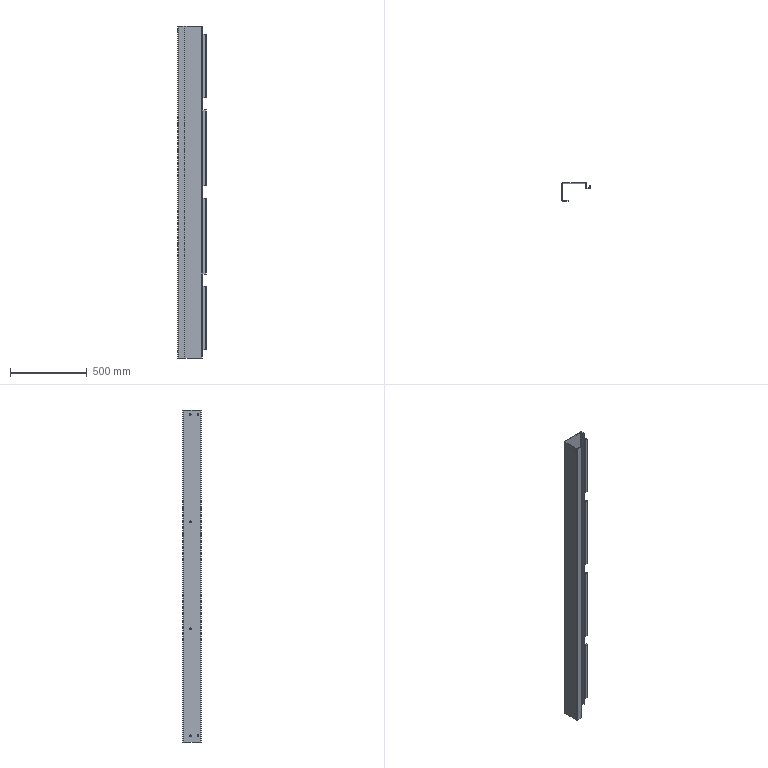Part | SolidWorks | features ICE 2, EdgeFlange 1, FlatPattern 1, LPattern 1, SMBaseFlange 1, SheetMetal 1 | 1 solid | 140 faces | box 184 x 120 x 2170 mm | volume 2431565 mm3 | plane 100 | cylinder 40 | commonest cylinder face diameters 7 x18 4 x11 10 x11